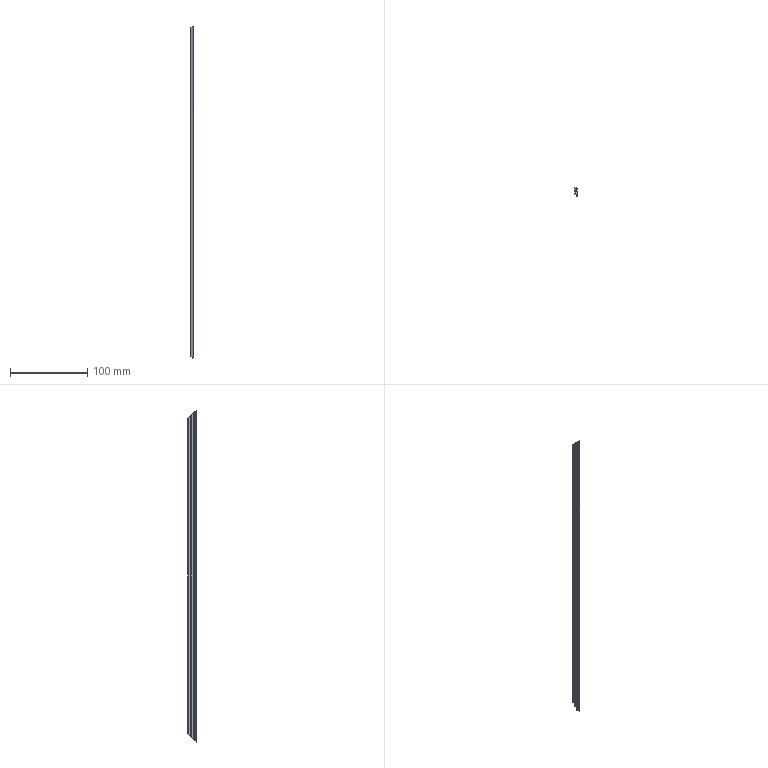Part | NX | features BREP 1 | 1 solid | 28 faces | box 3.587 x 11.224 x 429 mm | volume 9737 mm3 | plane 18 | cylinder 10 | commonest cylinder face diameters 0.4 x6 0.6 x2 1.942 x2
STEP:
#1=CARTESIAN_POINT('',(3.587,9.871,-204.628));
#2=VERTEX_POINT('',#1);
#3=CARTESIAN_POINT('',(3.287,9.567,-204.932));
#4=VERTEX_POINT('',#3);
#5=CARTESIAN_POINT('',(3.587,9.871,-204.628));
#6=CARTESIAN_POINT('',(3.589,9.693,-204.806));
#7=CARTESIAN_POINT('',(3.464,9.567,-204.932));
#8=CARTESIAN_POINT('',(3.287,9.567,-204.932));
#9=(BOUNDED_CURVE()B_SPLINE_CURVE(3,(#5,#6,#7,#8),.UNSPECIFIED.,.F.,.F.)B_SPLINE_CURVE_WITH_KNOTS((4,4),(4.699,6.283),.UNSPECIFIED.)CURVE()GEOMETRIC_REPRESENTATION_ITEM()RATIONAL_B_SPLINE_CURVE((1.,0.8015,0.8015,1.))REPRESENTATION_ITEM(''));
#10=EDGE_CURVE('',#2,#4,#9,.T.);
#11=ORIENTED_EDGE('',*,*,#10,.F.);
#12=CARTESIAN_POINT('',(3.587,9.871,204.628));
#13=VERTEX_POINT('',#12);
#14=CARTESIAN_POINT('',(3.587,9.871,214.5));
#15=DIRECTION('',(0.,0.,-1.));
#16=VECTOR('',#15,1000.);
#17=LINE('',#14,#16);
#18=EDGE_CURVE('',#13,#2,#17,.T.);
#19=ORIENTED_EDGE('',*,*,#18,.F.);
#20=CARTESIAN_POINT('',(3.287,9.567,204.932));
#21=VERTEX_POINT('',#20);
#22=CARTESIAN_POINT('',(3.287,9.567,204.932));
#23=CARTESIAN_POINT('',(3.464,9.567,204.932));
#24=CARTESIAN_POINT('',(3.589,9.693,204.806));
#25=CARTESIAN_POINT('',(3.587,9.871,204.628));
#26=(BOUNDED_CURVE()B_SPLINE_CURVE(3,(#22,#23,#24,#25),.UNSPECIFIED.,.F.,.F.)B_SPLINE_CURVE_WITH_KNOTS((4,4),(3.142,4.726),.UNSPECIFIED.)CURVE()GEOMETRIC_REPRESENTATION_ITEM()RATIONAL_B_SPLINE_CURVE((1.,0.8015,0.8015,1.))REPRESENTATION_ITEM(''));
#27=EDGE_CURVE('',#21,#13,#26,.T.);
#28=ORIENTED_EDGE('',*,*,#27,.F.);
#29=CARTESIAN_POINT('',(3.287,9.567,214.5));
#30=DIRECTION('',(0.,0.,-1.));
#31=VECTOR('',#30,1000.);
#32=LINE('',#29,#31);
#33=EDGE_CURVE('',#21,#4,#32,.T.);
#34=ORIENTED_EDGE('',*,*,#33,.T.);
#35=EDGE_LOOP('',(#11,#19,#28,#34));
#36=FACE_BOUND('',#35,.T.);
#37=CARTESIAN_POINT('',(3.287,9.867,214.5));
#38=DIRECTION('',(0.,0.,-1.));
#39=DIRECTION('',(-1.,0.,0.));
#40=AXIS2_PLACEMENT_3D('',#37,#38,#39);
#41=CYLINDRICAL_SURFACE('',#40,0.3);
#42=ADVANCED_FACE('',(#36),#41,.T.);
#43=CARTESIAN_POINT('',(3.447,10.36,-204.139));
#44=VERTEX_POINT('',#43);
#45=CARTESIAN_POINT('',(3.447,10.36,-204.139));
#46=CARTESIAN_POINT('',(3.536,10.211,-204.288));
#47=CARTESIAN_POINT('',(3.584,10.044,-204.455));
#48=CARTESIAN_POINT('',(3.587,9.871,-204.628));
#49=(BOUNDED_CURVE()B_SPLINE_CURVE(3,(#45,#46,#47,#48),.UNSPECIFIED.,.F.,.F.)B_SPLINE_CURVE_WITH_KNOTS((4,4),(4.169,4.699),.UNSPECIFIED.)CURVE()GEOMETRIC_REPRESENTATION_ITEM()RATIONAL_B_SPLINE_CURVE((1.,0.9767,0.9767,1.))REPRESENTATION_ITEM(''));
#50=EDGE_CURVE('',#44,#2,#49,.T.);
#51=ORIENTED_EDGE('',*,*,#50,.F.);
#52=CARTESIAN_POINT('',(3.447,10.36,204.139));
#53=VERTEX_POINT('',#52);
#54=CARTESIAN_POINT('',(3.447,10.36,214.5));
#55=DIRECTION('',(0.,0.,-1.));
#56=VECTOR('',#55,1000.);
#57=LINE('',#54,#56);
#58=EDGE_CURVE('',#53,#44,#57,.T.);
#59=ORIENTED_EDGE('',*,*,#58,.F.);
#60=CARTESIAN_POINT('',(3.587,9.871,204.628));
#61=CARTESIAN_POINT('',(3.584,10.044,204.455));
#62=CARTESIAN_POINT('',(3.536,10.211,204.288));
#63=CARTESIAN_POINT('',(3.447,10.36,204.139));
#64=(BOUNDED_CURVE()B_SPLINE_CURVE(3,(#60,#61,#62,#63),.UNSPECIFIED.,.F.,.F.)B_SPLINE_CURVE_WITH_KNOTS((4,4),(4.726,5.256),.UNSPECIFIED.)CURVE()GEOMETRIC_REPRESENTATION_ITEM()RATIONAL_B_SPLINE_CURVE((1.,0.9767,0.9767,1.))REPRESENTATION_ITEM(''));
#65=EDGE_CURVE('',#13,#53,#64,.T.);
#66=ORIENTED_EDGE('',*,*,#65,.F.);
#67=ORIENTED_EDGE('',*,*,#18,.T.);
#68=EDGE_LOOP('',(#51,#59,#66,#67));
#69=FACE_BOUND('',#68,.T.);
#70=CARTESIAN_POINT('',(2.616,9.857,214.5));
#71=DIRECTION('',(0.,0.,-1.));
#72=DIRECTION('',(-1.,0.,0.));
#73=AXIS2_PLACEMENT_3D('',#70,#71,#72);
#74=CYLINDRICAL_SURFACE('',#73,0.971);
#75=ADVANCED_FACE('',(#69),#74,.T.);
#76=CARTESIAN_POINT('',(0.2517,11.216,-203.283));
#77=VERTEX_POINT('',#76);
#78=CARTESIAN_POINT('',(-94.616,36.626,-177.873));
#79=DIRECTION('',(0.9352,-0.2505,-0.2505));
#80=VECTOR('',#79,1000.);
#81=LINE('',#78,#80);
#82=EDGE_CURVE('',#77,#44,#81,.T.);
#83=ORIENTED_EDGE('',*,*,#82,.F.);
#84=CARTESIAN_POINT('',(0.2517,11.216,203.283));
#85=VERTEX_POINT('',#84);
#86=CARTESIAN_POINT('',(0.2517,11.216,214.5));
#87=DIRECTION('',(0.,0.,-1.));
#88=VECTOR('',#87,1000.);
#89=LINE('',#86,#88);
#90=EDGE_CURVE('',#85,#77,#89,.T.);
#91=ORIENTED_EDGE('',*,*,#90,.F.);
#92=CARTESIAN_POINT('',(5.874,9.71,204.789));
#93=DIRECTION('',(-0.9352,0.2505,-0.2505));
#94=VECTOR('',#93,1000.);
#95=LINE('',#92,#94);
#96=EDGE_CURVE('',#53,#85,#95,.T.);
#97=ORIENTED_EDGE('',*,*,#96,.F.);
#98=ORIENTED_EDGE('',*,*,#58,.T.);
#99=EDGE_LOOP('',(#83,#91,#97,#98));
#100=FACE_BOUND('',#99,.T.);
#101=CARTESIAN_POINT('',(3.447,10.36,214.5));
#102=DIRECTION('',(-0.2587,-0.9659,0.));
#103=DIRECTION('',(-0.9659,0.2587,0.));
#104=AXIS2_PLACEMENT_3D('',#101,#102,#103);
#105=PLANE('',#104);
#106=ADVANCED_FACE('',(#100),#105,.F.);
#107=CARTESIAN_POINT('',(0.,11.022,-203.476));
#108=VERTEX_POINT('',#107);
#109=CARTESIAN_POINT('',(0.,11.022,-203.476));
#110=CARTESIAN_POINT('',(0.,11.165,-203.333));
#111=CARTESIAN_POINT('',(0.1135,11.253,-203.246));
#112=CARTESIAN_POINT('',(0.2517,11.216,-203.283));
#113=(BOUNDED_CURVE()B_SPLINE_CURVE(3,(#109,#110,#111,#112),.UNSPECIFIED.,.F.,.F.)B_SPLINE_CURVE_WITH_KNOTS((4,4),(1.571,3.403),.UNSPECIFIED.)CURVE()GEOMETRIC_REPRESENTATION_ITEM()RATIONAL_B_SPLINE_CURVE((1.,0.7392,0.7392,1.))REPRESENTATION_ITEM(''));
#114=EDGE_CURVE('',#108,#77,#113,.T.);
#115=ORIENTED_EDGE('',*,*,#114,.F.);
#116=CARTESIAN_POINT('',(0.,11.022,203.476));
#117=VERTEX_POINT('',#116);
#118=CARTESIAN_POINT('',(0.,11.022,214.5));
#119=DIRECTION('',(0.,0.,-1.));
#120=VECTOR('',#119,1000.);
#121=LINE('',#118,#120);
#122=EDGE_CURVE('',#117,#108,#121,.T.);
#123=ORIENTED_EDGE('',*,*,#122,.F.);
#124=CARTESIAN_POINT('',(0.2517,11.216,203.283));
#125=CARTESIAN_POINT('',(0.1135,11.253,203.246));
#126=CARTESIAN_POINT('',(0.,11.165,203.333));
#127=CARTESIAN_POINT('',(0.,11.022,203.476));
#128=(BOUNDED_CURVE()B_SPLINE_CURVE(3,(#124,#125,#126,#127),.UNSPECIFIED.,.F.,.F.)B_SPLINE_CURVE_WITH_KNOTS((4,4),(6.021,7.854),.UNSPECIFIED.)CURVE()GEOMETRIC_REPRESENTATION_ITEM()RATIONAL_B_SPLINE_CURVE((1.,0.7392,0.7392,1.))REPRESENTATION_ITEM(''));
#129=EDGE_CURVE('',#85,#117,#128,.T.);
#130=ORIENTED_EDGE('',*,*,#129,.F.);
#131=ORIENTED_EDGE('',*,*,#90,.T.);
#132=EDGE_LOOP('',(#115,#123,#130,#131));
#133=FACE_BOUND('',#132,.T.);
#134=CARTESIAN_POINT('',(0.2,11.022,214.5));
#135=DIRECTION('',(0.,0.,-1.));
#136=DIRECTION('',(-1.,0.,0.));
#137=AXIS2_PLACEMENT_3D('',#134,#135,#136);
#138=CYLINDRICAL_SURFACE('',#137,0.2);
#139=ADVANCED_FACE('',(#133),#138,.T.);
#140=CARTESIAN_POINT('',(0.,10.432,-204.067));
#141=VERTEX_POINT('',#140);
#142=CARTESIAN_POINT('',(0.,220.011,5.512));
#143=DIRECTION('',(0.,0.7071,0.7071));
#144=VECTOR('',#143,1000.);
#145=LINE('',#142,#144);
#146=EDGE_CURVE('',#141,#108,#145,.T.);
#147=ORIENTED_EDGE('',*,*,#146,.F.);
#148=CARTESIAN_POINT('',(0.,10.432,204.067));
#149=VERTEX_POINT('',#148);
#150=CARTESIAN_POINT('',(0.,10.432,214.5));
#151=DIRECTION('',(0.,0.,-1.));
#152=VECTOR('',#151,1000.);
#153=LINE('',#150,#152);
#154=EDGE_CURVE('',#149,#141,#153,.T.);
#155=ORIENTED_EDGE('',*,*,#154,.F.);
#156=CARTESIAN_POINT('',(0.,5.511,208.988));
#157=DIRECTION('',(0.,-0.7071,0.7071));
#158=VECTOR('',#157,1000.);
#159=LINE('',#156,#158);
#160=EDGE_CURVE('',#117,#149,#159,.T.);
#161=ORIENTED_EDGE('',*,*,#160,.F.);
#162=ORIENTED_EDGE('',*,*,#122,.T.);
#163=EDGE_LOOP('',(#147,#155,#161,#162));
#164=FACE_BOUND('',#163,.T.);
#165=CARTESIAN_POINT('',(0.,11.022,214.5));
#166=DIRECTION('',(1.,0.,0.));
#167=DIRECTION('',(0.,1.,0.));
#168=AXIS2_PLACEMENT_3D('',#165,#166,#167);
#169=PLANE('',#168);
#170=ADVANCED_FACE('',(#164),#169,.F.);
#171=CARTESIAN_POINT('',(0.1483,10.238,-204.26));
#172=VERTEX_POINT('',#171);
#173=CARTESIAN_POINT('',(0.1483,10.238,-204.26));
#174=CARTESIAN_POINT('',(0.05733,10.263,-204.236));
#175=CARTESIAN_POINT('',(0.,10.338,-204.161));
#176=CARTESIAN_POINT('',(0.,10.432,-204.067));
#177=(BOUNDED_CURVE()B_SPLINE_CURVE(3,(#173,#174,#175,#176),.UNSPECIFIED.,.F.,.F.)B_SPLINE_CURVE_WITH_KNOTS((4,4),(0.2616,1.571),.UNSPECIFIED.)CURVE()GEOMETRIC_REPRESENTATION_ITEM()RATIONAL_B_SPLINE_CURVE((1.,0.8622,0.8622,1.))REPRESENTATION_ITEM(''));
#178=EDGE_CURVE('',#172,#141,#177,.T.);
#179=ORIENTED_EDGE('',*,*,#178,.F.);
#180=CARTESIAN_POINT('',(0.1483,10.238,204.26));
#181=VERTEX_POINT('',#180);
#182=CARTESIAN_POINT('',(0.1483,10.238,214.5));
#183=DIRECTION('',(0.,0.,-1.));
#184=VECTOR('',#183,1000.);
#185=LINE('',#182,#184);
#186=EDGE_CURVE('',#181,#172,#185,.T.);
#187=ORIENTED_EDGE('',*,*,#186,.F.);
#188=CARTESIAN_POINT('',(0.,10.432,204.067));
#189=CARTESIAN_POINT('',(0.,10.338,204.161));
#190=CARTESIAN_POINT('',(0.05733,10.263,204.236));
#191=CARTESIAN_POINT('',(0.1483,10.238,204.26));
#192=(BOUNDED_CURVE()B_SPLINE_CURVE(3,(#188,#189,#190,#191),.UNSPECIFIED.,.F.,.F.)B_SPLINE_CURVE_WITH_KNOTS((4,4),(1.571,2.88),.UNSPECIFIED.)CURVE()GEOMETRIC_REPRESENTATION_ITEM()RATIONAL_B_SPLINE_CURVE((1.,0.8622,0.8622,1.))REPRESENTATION_ITEM(''));
#193=EDGE_CURVE('',#149,#181,#192,.T.);
#194=ORIENTED_EDGE('',*,*,#193,.F.);
#195=ORIENTED_EDGE('',*,*,#154,.T.);
#196=EDGE_LOOP('',(#179,#187,#194,#195));
#197=FACE_BOUND('',#196,.T.);
#198=CARTESIAN_POINT('',(0.2,10.432,214.5));
#199=DIRECTION('',(0.,0.,-1.));
#200=DIRECTION('',(-1.,0.,0.));
#201=AXIS2_PLACEMENT_3D('',#198,#199,#200);
#202=CYLINDRICAL_SURFACE('',#201,0.2);
#203=ADVANCED_FACE('',(#197),#202,.T.);
#204=CARTESIAN_POINT('',(0.854,10.05,-204.449));
#205=VERTEX_POINT('',#204);
#206=CARTESIAN_POINT('',(-97.905,36.489,-178.01));
#207=DIRECTION('',(-0.9352,0.2504,0.2504));
#208=VECTOR('',#207,1000.);
#209=LINE('',#206,#208);
#210=EDGE_CURVE('',#205,#172,#209,.T.);
#211=ORIENTED_EDGE('',*,*,#210,.F.);
#212=CARTESIAN_POINT('',(0.854,10.05,204.449));
#213=VERTEX_POINT('',#212);
#214=CARTESIAN_POINT('',(0.854,10.05,214.5));
#215=DIRECTION('',(0.,0.,-1.));
#216=VECTOR('',#215,1000.);
#217=LINE('',#214,#216);
#218=EDGE_CURVE('',#213,#205,#217,.T.);
#219=ORIENTED_EDGE('',*,*,#218,.F.);
#220=CARTESIAN_POINT('',(2.546,9.597,204.902));
#221=DIRECTION('',(0.9352,-0.2504,0.2504));
#222=VECTOR('',#221,1000.);
#223=LINE('',#220,#222);
#224=EDGE_CURVE('',#181,#213,#223,.T.);
#225=ORIENTED_EDGE('',*,*,#224,.F.);
#226=ORIENTED_EDGE('',*,*,#186,.T.);
#227=EDGE_LOOP('',(#211,#219,#225,#226));
#228=FACE_BOUND('',#227,.T.);
#229=CARTESIAN_POINT('',(0.1483,10.238,214.5));
#230=DIRECTION('',(0.2586,0.966,0.));
#231=DIRECTION('',(0.,0.,-1.));
#232=AXIS2_PLACEMENT_3D('',#229,#230,#231);
#233=PLANE('',#232);
#234=ADVANCED_FACE('',(#228),#233,.F.);
#235=CARTESIAN_POINT('',(1.256,6.926,-207.573));
#236=VERTEX_POINT('',#235);
#237=CARTESIAN_POINT('',(-25.866,217.806,3.307));
#238=DIRECTION('',(-0.09057,0.7042,0.7042));
#239=VECTOR('',#238,1000.);
#240=LINE('',#237,#239);
#241=EDGE_CURVE('',#236,#205,#240,.T.);
#242=ORIENTED_EDGE('',*,*,#241,.F.);
#243=CARTESIAN_POINT('',(1.256,6.926,207.573));
#244=VERTEX_POINT('',#243);
#245=CARTESIAN_POINT('',(1.256,6.926,214.5));
#246=DIRECTION('',(0.,0.,-1.));
#247=VECTOR('',#246,1000.);
#248=LINE('',#245,#247);
#249=EDGE_CURVE('',#244,#236,#248,.T.);
#250=ORIENTED_EDGE('',*,*,#249,.F.);
#251=CARTESIAN_POINT('',(1.495,5.065,209.433));
#252=DIRECTION('',(0.09057,-0.7042,0.7042));
#253=VECTOR('',#252,1000.);
#254=LINE('',#251,#253);
#255=EDGE_CURVE('',#213,#244,#254,.T.);
#256=ORIENTED_EDGE('',*,*,#255,.F.);
#257=ORIENTED_EDGE('',*,*,#218,.T.);
#258=EDGE_LOOP('',(#242,#250,#256,#257));
#259=FACE_BOUND('',#258,.T.);
#260=CARTESIAN_POINT('',(0.854,10.05,214.5));
#261=DIRECTION('',(0.9918,0.1276,0.));
#262=DIRECTION('',(0.,0.,-1.));
#263=AXIS2_PLACEMENT_3D('',#260,#261,#262);
#264=PLANE('',#263);
#265=ADVANCED_FACE('',(#259),#264,.F.);
#266=CARTESIAN_POINT('',(0.2517,7.195,-207.304));
#267=VERTEX_POINT('',#266);
#268=CARTESIAN_POINT('',(-97.576,33.385,-181.113));
#269=DIRECTION('',(0.9352,-0.2504,-0.2504));
#270=VECTOR('',#269,1000.);
#271=LINE('',#268,#270);
#272=EDGE_CURVE('',#267,#236,#271,.T.);
#273=ORIENTED_EDGE('',*,*,#272,.F.);
#274=CARTESIAN_POINT('',(0.2517,7.195,207.304));
#275=VERTEX_POINT('',#274);
#276=CARTESIAN_POINT('',(0.2517,7.195,214.5));
#277=DIRECTION('',(0.,0.,-1.));
#278=VECTOR('',#277,1000.);
#279=LINE('',#276,#278);
#280=EDGE_CURVE('',#275,#267,#279,.T.);
#281=ORIENTED_EDGE('',*,*,#280,.F.);
#282=CARTESIAN_POINT('',(2.878,6.492,208.007));
#283=DIRECTION('',(-0.9352,0.2504,-0.2504));
#284=VECTOR('',#283,1000.);
#285=LINE('',#282,#284);
#286=EDGE_CURVE('',#244,#275,#285,.T.);
#287=ORIENTED_EDGE('',*,*,#286,.F.);
#288=ORIENTED_EDGE('',*,*,#249,.T.);
#289=EDGE_LOOP('',(#273,#281,#287,#288));
#290=FACE_BOUND('',#289,.T.);
#291=CARTESIAN_POINT('',(1.256,6.926,214.5));
#292=DIRECTION('',(-0.2586,-0.966,0.));
#293=DIRECTION('',(-0.966,0.2586,0.));
#294=AXIS2_PLACEMENT_3D('',#291,#292,#293);
#295=PLANE('',#294);
#296=ADVANCED_FACE('',(#290),#295,.F.);
#297=CARTESIAN_POINT('',(0.,7.001,-207.497));
#298=VERTEX_POINT('',#297);
#299=CARTESIAN_POINT('',(0.,7.001,-207.497));
#300=CARTESIAN_POINT('',(0.,7.145,-207.354));
#301=CARTESIAN_POINT('',(0.1135,7.232,-207.267));
#302=CARTESIAN_POINT('',(0.2517,7.195,-207.304));
#303=(BOUNDED_CURVE()B_SPLINE_CURVE(3,(#299,#300,#301,#302),.UNSPECIFIED.,.F.,.F.)B_SPLINE_CURVE_WITH_KNOTS((4,4),(1.571,3.403),.UNSPECIFIED.)CURVE()GEOMETRIC_REPRESENTATION_ITEM()RATIONAL_B_SPLINE_CURVE((1.,0.7392,0.7392,1.))REPRESENTATION_ITEM(''));
#304=EDGE_CURVE('',#298,#267,#303,.T.);
#305=ORIENTED_EDGE('',*,*,#304,.F.);
#306=CARTESIAN_POINT('',(0.,7.001,207.497));
#307=VERTEX_POINT('',#306);
#308=CARTESIAN_POINT('',(0.,7.001,214.5));
#309=DIRECTION('',(0.,0.,-1.));
#310=VECTOR('',#309,1000.);
#311=LINE('',#308,#310);
#312=EDGE_CURVE('',#307,#298,#311,.T.);
#313=ORIENTED_EDGE('',*,*,#312,.F.);
#314=CARTESIAN_POINT('',(0.2517,7.195,207.304));
#315=CARTESIAN_POINT('',(0.1135,7.232,207.267));
#316=CARTESIAN_POINT('',(0.,7.145,207.354));
#317=CARTESIAN_POINT('',(0.,7.001,207.497));
#318=(BOUNDED_CURVE()B_SPLINE_CURVE(3,(#314,#315,#316,#317),.UNSPECIFIED.,.F.,.F.)B_SPLINE_CURVE_WITH_KNOTS((4,4),(6.022,7.854),.UNSPECIFIED.)CURVE()GEOMETRIC_REPRESENTATION_ITEM()RATIONAL_B_SPLINE_CURVE((1.,0.7392,0.7392,1.))REPRESENTATION_ITEM(''));
#319=EDGE_CURVE('',#275,#307,#318,.T.);
#320=ORIENTED_EDGE('',*,*,#319,.F.);
#321=ORIENTED_EDGE('',*,*,#280,.T.);
#322=EDGE_LOOP('',(#305,#313,#320,#321));
#323=FACE_BOUND('',#322,.T.);
#324=CARTESIAN_POINT('',(0.2,7.001,214.5));
#325=DIRECTION('',(0.,0.,-1.));
#326=DIRECTION('',(-1.,0.,0.));
#327=AXIS2_PLACEMENT_3D('',#324,#325,#326);
#328=CYLINDRICAL_SURFACE('',#327,0.2);
#329=ADVANCED_FACE('',(#323),#328,.T.);
#330=CARTESIAN_POINT('',(0.,6.41,-208.089));
#331=VERTEX_POINT('',#330);
#332=CARTESIAN_POINT('',(0.,218.,3.501));
#333=DIRECTION('',(0.,0.7071,0.7071));
#334=VECTOR('',#333,1000.);
#335=LINE('',#332,#334);
#336=EDGE_CURVE('',#331,#298,#335,.T.);
#337=ORIENTED_EDGE('',*,*,#336,.F.);
#338=CARTESIAN_POINT('',(0.,6.41,208.089));
#339=VERTEX_POINT('',#338);
#340=CARTESIAN_POINT('',(0.,6.41,214.5));
#341=DIRECTION('',(0.,0.,-1.));
#342=VECTOR('',#341,1000.);
#343=LINE('',#340,#342);
#344=EDGE_CURVE('',#339,#331,#343,.T.);
#345=ORIENTED_EDGE('',*,*,#344,.F.);
#346=CARTESIAN_POINT('',(0.,3.5,210.999));
#347=DIRECTION('',(0.,-0.7071,0.7071));
#348=VECTOR('',#347,1000.);
#349=LINE('',#346,#348);
#350=EDGE_CURVE('',#307,#339,#349,.T.);
#351=ORIENTED_EDGE('',*,*,#350,.F.);
#352=ORIENTED_EDGE('',*,*,#312,.T.);
#353=EDGE_LOOP('',(#337,#345,#351,#352));
#354=FACE_BOUND('',#353,.T.);
#355=CARTESIAN_POINT('',(0.,7.001,214.5));
#356=DIRECTION('',(1.,0.,0.));
#357=DIRECTION('',(0.,1.,0.));
#358=AXIS2_PLACEMENT_3D('',#355,#356,#357);
#359=PLANE('',#358);
#360=ADVANCED_FACE('',(#354),#359,.F.);
#361=CARTESIAN_POINT('',(0.1482,6.217,-208.282));
#362=VERTEX_POINT('',#361);
#363=CARTESIAN_POINT('',(0.1482,6.217,-208.282));
#364=CARTESIAN_POINT('',(0.0573,6.241,-208.258));
#365=CARTESIAN_POINT('',(0.,6.316,-208.183));
#366=CARTESIAN_POINT('',(0.,6.41,-208.089));
#367=(BOUNDED_CURVE()B_SPLINE_CURVE(3,(#363,#364,#365,#366),.UNSPECIFIED.,.F.,.F.)B_SPLINE_CURVE_WITH_KNOTS((4,4),(0.2619,1.571),.UNSPECIFIED.)CURVE()GEOMETRIC_REPRESENTATION_ITEM()RATIONAL_B_SPLINE_CURVE((1.,0.8623,0.8623,1.))REPRESENTATION_ITEM(''));
#368=EDGE_CURVE('',#362,#331,#367,.T.);
#369=ORIENTED_EDGE('',*,*,#368,.F.);
#370=CARTESIAN_POINT('',(0.1482,6.217,208.282));
#371=VERTEX_POINT('',#370);
#372=CARTESIAN_POINT('',(0.1482,6.217,214.5));
#373=DIRECTION('',(0.,0.,-1.));
#374=VECTOR('',#373,1000.);
#375=LINE('',#372,#374);
#376=EDGE_CURVE('',#371,#362,#375,.T.);
#377=ORIENTED_EDGE('',*,*,#376,.F.);
#378=CARTESIAN_POINT('',(0.,6.41,208.089));
#379=CARTESIAN_POINT('',(0.,6.316,208.183));
#380=CARTESIAN_POINT('',(0.0573,6.241,208.258));
#381=CARTESIAN_POINT('',(0.1482,6.217,208.282));
#382=(BOUNDED_CURVE()B_SPLINE_CURVE(3,(#378,#379,#380,#381),.UNSPECIFIED.,.F.,.F.)B_SPLINE_CURVE_WITH_KNOTS((4,4),(1.571,2.88),.UNSPECIFIED.)CURVE()GEOMETRIC_REPRESENTATION_ITEM()RATIONAL_B_SPLINE_CURVE((1.,0.8623,0.8623,1.))REPRESENTATION_ITEM(''));
#383=EDGE_CURVE('',#339,#371,#382,.T.);
#384=ORIENTED_EDGE('',*,*,#383,.F.);
#385=ORIENTED_EDGE('',*,*,#344,.T.);
#386=EDGE_LOOP('',(#369,#377,#384,#385));
#387=FACE_BOUND('',#386,.T.);
#388=CARTESIAN_POINT('',(0.2,6.41,214.5));
#389=DIRECTION('',(0.,0.,-1.));
#390=DIRECTION('',(-1.,0.,0.));
#391=AXIS2_PLACEMENT_3D('',#388,#389,#390);
#392=CYLINDRICAL_SURFACE('',#391,0.2);
#393=ADVANCED_FACE('',(#387),#392,.T.);
#394=CARTESIAN_POINT('',(1.39,5.884,-208.615));
#395=VERTEX_POINT('',#394);
#396=CARTESIAN_POINT('',(-98.949,32.783,-181.716));
#397=DIRECTION('',(-0.9351,0.2507,0.2507));
#398=VECTOR('',#397,1000.);
#399=LINE('',#396,#398);
#400=EDGE_CURVE('',#395,#362,#399,.T.);
#401=ORIENTED_EDGE('',*,*,#400,.F.);
#402=CARTESIAN_POINT('',(1.39,5.884,208.615));
#403=VERTEX_POINT('',#402);
#404=CARTESIAN_POINT('',(1.39,5.884,214.5));
#405=DIRECTION('',(0.,0.,-1.));
#406=VECTOR('',#405,1000.);
#407=LINE('',#404,#406);
#408=EDGE_CURVE('',#403,#395,#407,.T.);
#409=ORIENTED_EDGE('',*,*,#408,.F.);
#410=CARTESIAN_POINT('',(1.606,5.826,208.673));
#411=DIRECTION('',(0.9351,-0.2507,0.2507));
#412=VECTOR('',#411,1000.);
#413=LINE('',#410,#412);
#414=EDGE_CURVE('',#371,#403,#413,.T.);
#415=ORIENTED_EDGE('',*,*,#414,.F.);
#416=ORIENTED_EDGE('',*,*,#376,.T.);
#417=EDGE_LOOP('',(#401,#409,#415,#416));
#418=FACE_BOUND('',#417,.T.);
#419=CARTESIAN_POINT('',(0.1482,6.217,214.5));
#420=DIRECTION('',(0.2589,0.9659,0.));
#421=DIRECTION('',(0.,0.,-1.));
#422=AXIS2_PLACEMENT_3D('',#419,#420,#421);
#423=PLANE('',#422);
#424=ADVANCED_FACE('',(#418),#423,.F.);
#425=CARTESIAN_POINT('',(1.791,2.761,-211.738));
#426=VERTEX_POINT('',#425);
#427=CARTESIAN_POINT('',(-25.595,215.706,1.207));
#428=DIRECTION('',(-0.09057,0.7042,0.7042));
#429=VECTOR('',#428,1000.);
#430=LINE('',#427,#429);
#431=EDGE_CURVE('',#426,#395,#430,.T.);
#432=ORIENTED_EDGE('',*,*,#431,.F.);
#433=CARTESIAN_POINT('',(1.791,2.761,211.738));
#434=VERTEX_POINT('',#433);
#435=CARTESIAN_POINT('',(1.791,2.761,214.5));
#436=DIRECTION('',(0.,0.,-1.));
#437=VECTOR('',#436,1000.);
#438=LINE('',#435,#437);
#439=EDGE_CURVE('',#434,#426,#438,.T.);
#440=ORIENTED_EDGE('',*,*,#439,.F.);
#441=CARTESIAN_POINT('',(1.765,2.965,211.533));
#442=DIRECTION('',(0.09057,-0.7042,0.7042));
#443=VECTOR('',#442,1000.);
#444=LINE('',#441,#443);
#445=EDGE_CURVE('',#403,#434,#444,.T.);
#446=ORIENTED_EDGE('',*,*,#445,.F.);
#447=ORIENTED_EDGE('',*,*,#408,.T.);
#448=EDGE_LOOP('',(#432,#440,#446,#447));
#449=FACE_BOUND('',#448,.T.);
#450=CARTESIAN_POINT('',(1.39,5.884,214.5));
#451=DIRECTION('',(0.9918,0.1276,0.));
#452=DIRECTION('',(0.,0.,-1.));
#453=AXIS2_PLACEMENT_3D('',#450,#451,#452);
#454=PLANE('',#453);
#455=ADVANCED_FACE('',(#449),#454,.F.);
#456=CARTESIAN_POINT('',(0.2518,3.174,-211.325));
#457=VERTEX_POINT('',#456);
#458=CARTESIAN_POINT('',(-98.108,29.54,-184.959));
#459=DIRECTION('',(0.9351,-0.2506,-0.2506));
#460=VECTOR('',#459,1000.);
#461=LINE('',#458,#460);
#462=EDGE_CURVE('',#457,#426,#461,.T.);
#463=ORIENTED_EDGE('',*,*,#462,.F.);
#464=CARTESIAN_POINT('',(0.2518,3.174,211.325));
#465=VERTEX_POINT('',#464);
#466=CARTESIAN_POINT('',(0.2518,3.174,214.5));
#467=DIRECTION('',(0.,0.,-1.));
#468=VECTOR('',#467,1000.);
#469=LINE('',#466,#468);
#470=EDGE_CURVE('',#465,#457,#469,.T.);
#471=ORIENTED_EDGE('',*,*,#470,.F.);
#472=CARTESIAN_POINT('',(2.439,2.588,211.911));
#473=DIRECTION('',(-0.9351,0.2506,-0.2506));
#474=VECTOR('',#473,1000.);
#475=LINE('',#472,#474);
#476=EDGE_CURVE('',#434,#465,#475,.T.);
#477=ORIENTED_EDGE('',*,*,#476,.F.);
#478=ORIENTED_EDGE('',*,*,#439,.T.);
#479=EDGE_LOOP('',(#463,#471,#477,#478));
#480=FACE_BOUND('',#479,.T.);
#481=CARTESIAN_POINT('',(1.791,2.761,214.5));
#482=DIRECTION('',(-0.2589,-0.9659,0.));
#483=DIRECTION('',(-0.9659,0.2589,0.));
#484=AXIS2_PLACEMENT_3D('',#481,#482,#483);
#485=PLANE('',#484);
#486=ADVANCED_FACE('',(#480),#485,.F.);
#487=CARTESIAN_POINT('',(0.,2.981,-211.518));
#488=VERTEX_POINT('',#487);
#489=CARTESIAN_POINT('',(0.,2.981,-211.518));
#490=CARTESIAN_POINT('',(0.,3.124,-211.375));
#491=CARTESIAN_POINT('',(0.1135,3.211,-211.288));
#492=CARTESIAN_POINT('',(0.2518,3.174,-211.325));
#493=(BOUNDED_CURVE()B_SPLINE_CURVE(3,(#489,#490,#491,#492),.UNSPECIFIED.,.F.,.F.)B_SPLINE_CURVE_WITH_KNOTS((4,4),(1.571,3.403),.UNSPECIFIED.)CURVE()GEOMETRIC_REPRESENTATION_ITEM()RATIONAL_B_SPLINE_CURVE((1.,0.7391,0.7391,1.))REPRESENTATION_ITEM(''));
#494=EDGE_CURVE('',#488,#457,#493,.T.);
#495=ORIENTED_EDGE('',*,*,#494,.F.);
#496=CARTESIAN_POINT('',(0.,2.981,211.518));
#497=VERTEX_POINT('',#496);
#498=CARTESIAN_POINT('',(0.,2.981,214.5));
#499=DIRECTION('',(0.,0.,-1.));
#500=VECTOR('',#499,1000.);
#501=LINE('',#498,#500);
#502=EDGE_CURVE('',#497,#488,#501,.T.);
#503=ORIENTED_EDGE('',*,*,#502,.F.);
#504=CARTESIAN_POINT('',(0.2518,3.174,211.325));
#505=CARTESIAN_POINT('',(0.1135,3.211,211.288));
#506=CARTESIAN_POINT('',(0.,3.124,211.375));
#507=CARTESIAN_POINT('',(0.,2.981,211.518));
#508=(BOUNDED_CURVE()B_SPLINE_CURVE(3,(#504,#505,#506,#507),.UNSPECIFIED.,.F.,.F.)B_SPLINE_CURVE_WITH_KNOTS((4,4),(6.021,7.854),.UNSPECIFIED.)CURVE()GEOMETRIC_REPRESENTATION_ITEM()RATIONAL_B_SPLINE_CURVE((1.,0.7391,0.7391,1.))REPRESENTATION_ITEM(''));
#509=EDGE_CURVE('',#465,#497,#508,.T.);
#510=ORIENTED_EDGE('',*,*,#509,.F.);
#511=ORIENTED_EDGE('',*,*,#470,.T.);
#512=EDGE_LOOP('',(#495,#503,#510,#511));
#513=FACE_BOUND('',#512,.T.);
#514=CARTESIAN_POINT('',(0.2,2.981,214.5));
#515=DIRECTION('',(0.,0.,-1.));
#516=DIRECTION('',(-1.,0.,0.));
#517=AXIS2_PLACEMENT_3D('',#514,#515,#516);
#518=CYLINDRICAL_SURFACE('',#517,0.2);
#519=ADVANCED_FACE('',(#513),#518,.T.);
#520=CARTESIAN_POINT('',(0.,2.39,-212.109));
#521=VERTEX_POINT('',#520);
#522=CARTESIAN_POINT('',(0.,215.99,1.491));
#523=DIRECTION('',(0.,0.7071,0.7071));
#524=VECTOR('',#523,1000.);
#525=LINE('',#522,#524);
#526=EDGE_CURVE('',#521,#488,#525,.T.);
#527=ORIENTED_EDGE('',*,*,#526,.F.);
#528=CARTESIAN_POINT('',(0.,2.39,212.109));
#529=VERTEX_POINT('',#528);
#530=CARTESIAN_POINT('',(0.,2.39,214.5));
#531=DIRECTION('',(0.,0.,-1.));
#532=VECTOR('',#531,1000.);
#533=LINE('',#530,#532);
#534=EDGE_CURVE('',#529,#521,#533,.T.);
#535=ORIENTED_EDGE('',*,*,#534,.F.);
#536=CARTESIAN_POINT('',(0.,1.49,213.009));
#537=DIRECTION('',(0.,-0.7071,0.7071));
#538=VECTOR('',#537,1000.);
#539=LINE('',#536,#538);
#540=EDGE_CURVE('',#497,#529,#539,.T.);
#541=ORIENTED_EDGE('',*,*,#540,.F.);
#542=ORIENTED_EDGE('',*,*,#502,.T.);
#543=EDGE_LOOP('',(#527,#535,#541,#542));
#544=FACE_BOUND('',#543,.T.);
#545=CARTESIAN_POINT('',(0.,2.981,214.5));
#546=DIRECTION('',(1.,0.,0.));
#547=DIRECTION('',(0.,1.,0.));
#548=AXIS2_PLACEMENT_3D('',#545,#546,#547);
#549=PLANE('',#548);
#550=ADVANCED_FACE('',(#544),#549,.F.);
#551=CARTESIAN_POINT('',(0.1482,2.196,-212.302));
#552=VERTEX_POINT('',#551);
#553=CARTESIAN_POINT('',(0.1482,2.196,-212.302));
#554=CARTESIAN_POINT('',(0.05729,2.221,-212.278));
#555=CARTESIAN_POINT('',(0.,2.295,-212.203));
#556=CARTESIAN_POINT('',(0.,2.39,-212.109));
#557=(BOUNDED_CURVE()B_SPLINE_CURVE(3,(#553,#554,#555,#556),.UNSPECIFIED.,.F.,.F.)B_SPLINE_CURVE_WITH_KNOTS((4,4),(0.262,1.571),.UNSPECIFIED.)CURVE()GEOMETRIC_REPRESENTATION_ITEM()RATIONAL_B_SPLINE_CURVE((1.,0.8623,0.8623,1.))REPRESENTATION_ITEM(''));
#558=EDGE_CURVE('',#552,#521,#557,.T.);
#559=ORIENTED_EDGE('',*,*,#558,.F.);
#560=CARTESIAN_POINT('',(0.1482,2.196,212.302));
#561=VERTEX_POINT('',#560);
#562=CARTESIAN_POINT('',(0.1482,2.196,214.5));
#563=DIRECTION('',(0.,0.,-1.));
#564=VECTOR('',#563,1000.);
#565=LINE('',#562,#564);
#566=EDGE_CURVE('',#561,#552,#565,.T.);
#567=ORIENTED_EDGE('',*,*,#566,.F.);
#568=CARTESIAN_POINT('',(0.,2.39,212.109));
#569=CARTESIAN_POINT('',(0.,2.295,212.203));
#570=CARTESIAN_POINT('',(0.05729,2.221,212.278));
#571=CARTESIAN_POINT('',(0.1482,2.196,212.302));
#572=(BOUNDED_CURVE()B_SPLINE_CURVE(3,(#568,#569,#570,#571),.UNSPECIFIED.,.F.,.F.)B_SPLINE_CURVE_WITH_KNOTS((4,4),(1.571,2.88),.UNSPECIFIED.)CURVE()GEOMETRIC_REPRESENTATION_ITEM()RATIONAL_B_SPLINE_CURVE((1.,0.8623,0.8623,1.))REPRESENTATION_ITEM(''));
#573=EDGE_CURVE('',#529,#561,#572,.T.);
#574=ORIENTED_EDGE('',*,*,#573,.F.);
#575=ORIENTED_EDGE('',*,*,#534,.T.);
#576=EDGE_LOOP('',(#559,#567,#574,#575));
#577=FACE_BOUND('',#576,.T.);
#578=CARTESIAN_POINT('',(0.2,2.39,214.5));
#579=DIRECTION('',(0.,0.,-1.));
#580=DIRECTION('',(-1.,0.,0.));
#581=AXIS2_PLACEMENT_3D('',#578,#579,#580);
#582=CYLINDRICAL_SURFACE('',#581,0.2);
#583=ADVANCED_FACE('',(#577),#582,.T.);
#584=CARTESIAN_POINT('',(1.925,1.72,-212.779));
#585=VERTEX_POINT('',#584);
#586=CARTESIAN_POINT('',(-99.901,29.022,-185.477));
#587=DIRECTION('',(-0.935,0.2507,0.2507));
#588=VECTOR('',#587,1000.);
#589=LINE('',#586,#588);
#590=EDGE_CURVE('',#585,#552,#589,.T.);
#591=ORIENTED_EDGE('',*,*,#590,.F.);
#592=CARTESIAN_POINT('',(1.925,1.72,212.779));
#593=VERTEX_POINT('',#592);
#594=CARTESIAN_POINT('',(1.925,1.72,214.5));
#595=DIRECTION('',(0.,0.,-1.));
#596=VECTOR('',#595,1000.);
#597=LINE('',#594,#596);
#598=EDGE_CURVE('',#593,#585,#597,.T.);
#599=ORIENTED_EDGE('',*,*,#598,.F.);
#600=CARTESIAN_POINT('',(0.6633,2.058,212.441));
#601=DIRECTION('',(0.935,-0.2507,0.2507));
#602=VECTOR('',#601,1000.);
#603=LINE('',#600,#602);
#604=EDGE_CURVE('',#561,#593,#603,.T.);
#605=ORIENTED_EDGE('',*,*,#604,.F.);
#606=ORIENTED_EDGE('',*,*,#566,.T.);
#607=EDGE_LOOP('',(#591,#599,#605,#606));
#608=FACE_BOUND('',#607,.T.);
#609=CARTESIAN_POINT('',(0.1482,2.196,214.5));
#610=DIRECTION('',(0.259,0.9659,0.));
#611=DIRECTION('',(0.,0.,-1.));
#612=AXIS2_PLACEMENT_3D('',#609,#610,#611);
#613=PLANE('',#612);
#614=ADVANCED_FACE('',(#608),#613,.F.);
#615=CARTESIAN_POINT('',(2.108,0.3017,-214.197));
#616=VERTEX_POINT('',#615);
#617=CARTESIAN_POINT('',(-25.326,213.607,-0.8918));
#618=DIRECTION('',(-0.09057,0.7042,0.7042));
#619=VECTOR('',#618,1000.);
#620=LINE('',#617,#619);
#621=EDGE_CURVE('',#616,#585,#620,.T.);
#622=ORIENTED_EDGE('',*,*,#621,.F.);
#623=CARTESIAN_POINT('',(2.108,0.3017,214.197));
#624=VERTEX_POINT('',#623);
#625=CARTESIAN_POINT('',(2.108,0.3017,214.5));
#626=DIRECTION('',(0.,0.,-1.));
#627=VECTOR('',#626,1000.);
#628=LINE('',#625,#627);
#629=EDGE_CURVE('',#624,#616,#628,.T.);
#630=ORIENTED_EDGE('',*,*,#629,.F.);
#631=CARTESIAN_POINT('',(2.035,0.8664,213.632));
#632=DIRECTION('',(0.09057,-0.7042,0.7042));
#633=VECTOR('',#632,1000.);
#634=LINE('',#631,#633);
#635=EDGE_CURVE('',#593,#624,#634,.T.);
#636=ORIENTED_EDGE('',*,*,#635,.F.);
#637=ORIENTED_EDGE('',*,*,#598,.T.);
#638=EDGE_LOOP('',(#622,#630,#636,#637));
#639=FACE_BOUND('',#638,.T.);
#640=CARTESIAN_POINT('',(1.925,1.72,214.5));
#641=DIRECTION('',(0.9918,0.1276,0.));
#642=DIRECTION('',(0.,0.,-1.));
#643=AXIS2_PLACEMENT_3D('',#640,#641,#642);
#644=PLANE('',#643);
#645=ADVANCED_FACE('',(#639),#644,.F.);
#646=ORIENTED_EDGE('',*,*,#629,.T.);
#647=CARTESIAN_POINT('',(3.447,0.2347,-214.264));
#648=VERTEX_POINT('',#647);
#649=CARTESIAN_POINT('',(3.447,0.2347,-214.264));
#650=CARTESIAN_POINT('',(3.032,-0.1233,-214.622));
#651=CARTESIAN_POINT('',(2.485,-0.0959,-214.595));
#652=CARTESIAN_POINT('',(2.108,0.3017,-214.197));
#653=(BOUNDED_CURVE()B_SPLINE_CURVE(3,(#649,#650,#651,#652),.UNSPECIFIED.,.F.,.F.)B_SPLINE_CURVE_WITH_KNOTS((4,4),(5.571,7.095),.UNSPECIFIED.)CURVE()GEOMETRIC_REPRESENTATION_ITEM()RATIONAL_B_SPLINE_CURVE((1.,0.8156,0.8156,1.))REPRESENTATION_ITEM(''));
#654=EDGE_CURVE('',#648,#616,#653,.T.);
#655=ORIENTED_EDGE('',*,*,#654,.F.);
#656=CARTESIAN_POINT('',(3.447,0.2347,214.264));
#657=VERTEX_POINT('',#656);
#658=CARTESIAN_POINT('',(3.447,0.2347,214.5));
#659=DIRECTION('',(0.,0.,-1.));
#660=VECTOR('',#659,1000.);
#661=LINE('',#658,#660);
#662=EDGE_CURVE('',#657,#648,#661,.T.);
#663=ORIENTED_EDGE('',*,*,#662,.F.);
#664=CARTESIAN_POINT('',(2.108,0.3017,214.197));
#665=CARTESIAN_POINT('',(2.485,-0.0959,214.595));
#666=CARTESIAN_POINT('',(3.032,-0.1233,214.622));
#667=CARTESIAN_POINT('',(3.447,0.2347,214.264));
#668=(BOUNDED_CURVE()B_SPLINE_CURVE(3,(#664,#665,#666,#667),.UNSPECIFIED.,.F.,.F.)B_SPLINE_CURVE_WITH_KNOTS((4,4),(2.33,3.854),.UNSPECIFIED.)CURVE()GEOMETRIC_REPRESENTATION_ITEM()RATIONAL_B_SPLINE_CURVE((1.,0.8156,0.8156,1.))REPRESENTATION_ITEM(''));
#669=EDGE_CURVE('',#624,#657,#668,.T.);
#670=ORIENTED_EDGE('',*,*,#669,.F.);
#671=EDGE_LOOP('',(#646,#655,#663,#670));
#672=FACE_BOUND('',#671,.T.);
#673=CARTESIAN_POINT('',(2.812,0.9697,214.5));
#674=DIRECTION('',(0.,0.,-1.));
#675=DIRECTION('',(-1.,0.,0.));
#676=AXIS2_PLACEMENT_3D('',#673,#674,#675);
#677=CYLINDRICAL_SURFACE('',#676,0.971);
#678=ADVANCED_FACE('',(#672),#677,.T.);
#679=CARTESIAN_POINT('',(3.447,5.067,-209.432));
#680=VERTEX_POINT('',#679);
#681=CARTESIAN_POINT('',(3.447,214.617,0.1179));
#682=DIRECTION('',(0.,-0.7071,-0.7071));
#683=VECTOR('',#682,1000.);
#684=LINE('',#681,#683);
#685=EDGE_CURVE('',#680,#648,#684,.T.);
#686=ORIENTED_EDGE('',*,*,#685,.F.);
#687=CARTESIAN_POINT('',(3.447,5.067,209.432));
#688=VERTEX_POINT('',#687);
#689=CARTESIAN_POINT('',(3.447,5.067,214.5));
#690=DIRECTION('',(0.,0.,-1.));
#691=VECTOR('',#690,1000.);
#692=LINE('',#689,#691);
#693=EDGE_CURVE('',#688,#680,#692,.T.);
#694=ORIENTED_EDGE('',*,*,#693,.F.);
#695=CARTESIAN_POINT('',(3.447,0.1167,214.382));
#696=DIRECTION('',(0.,0.7071,-0.7071));
#697=VECTOR('',#696,1000.);
#698=LINE('',#695,#697);
#699=EDGE_CURVE('',#657,#688,#698,.T.);
#700=ORIENTED_EDGE('',*,*,#699,.F.);
#701=ORIENTED_EDGE('',*,*,#662,.T.);
#702=EDGE_LOOP('',(#686,#694,#700,#701));
#703=FACE_BOUND('',#702,.T.);
#704=CARTESIAN_POINT('',(3.447,0.2347,214.5));
#705=DIRECTION('',(-1.,0.,0.));
#706=DIRECTION('',(0.,0.,1.));
#707=AXIS2_PLACEMENT_3D('',#704,#705,#706);
#708=PLANE('',#707);
#709=ADVANCED_FACE('',(#703),#708,.F.);
#710=CARTESIAN_POINT('',(3.147,5.367,-209.132));
#711=VERTEX_POINT('',#710);
#712=CARTESIAN_POINT('',(3.147,5.367,-209.132));
#713=CARTESIAN_POINT('',(3.322,5.367,-209.132));
#714=CARTESIAN_POINT('',(3.447,5.242,-209.256));
#715=CARTESIAN_POINT('',(3.447,5.067,-209.432));
#716=(BOUNDED_CURVE()B_SPLINE_CURVE(3,(#712,#713,#714,#715),.UNSPECIFIED.,.F.,.F.)B_SPLINE_CURVE_WITH_KNOTS((4,4),(3.142,4.712),.UNSPECIFIED.)CURVE()GEOMETRIC_REPRESENTATION_ITEM()RATIONAL_B_SPLINE_CURVE((1.,0.8047,0.8047,1.))REPRESENTATION_ITEM(''));
#717=EDGE_CURVE('',#711,#680,#716,.T.);
#718=ORIENTED_EDGE('',*,*,#717,.F.);
#719=CARTESIAN_POINT('',(3.147,5.367,209.132));
#720=VERTEX_POINT('',#719);
#721=CARTESIAN_POINT('',(3.147,5.367,214.5));
#722=DIRECTION('',(0.,0.,-1.));
#723=VECTOR('',#722,1000.);
#724=LINE('',#721,#723);
#725=EDGE_CURVE('',#720,#711,#724,.T.);
#726=ORIENTED_EDGE('',*,*,#725,.F.);
#727=CARTESIAN_POINT('',(3.447,5.067,209.432));
#728=CARTESIAN_POINT('',(3.447,5.242,209.256));
#729=CARTESIAN_POINT('',(3.322,5.367,209.132));
#730=CARTESIAN_POINT('',(3.147,5.367,209.132));
#731=(BOUNDED_CURVE()B_SPLINE_CURVE(3,(#727,#728,#729,#730),.UNSPECIFIED.,.F.,.F.)B_SPLINE_CURVE_WITH_KNOTS((4,4),(4.712,6.283),.UNSPECIFIED.)CURVE()GEOMETRIC_REPRESENTATION_ITEM()RATIONAL_B_SPLINE_CURVE((1.,0.8047,0.8047,1.))REPRESENTATION_ITEM(''));
#732=EDGE_CURVE('',#688,#720,#731,.T.);
#733=ORIENTED_EDGE('',*,*,#732,.F.);
#734=ORIENTED_EDGE('',*,*,#693,.T.);
#735=EDGE_LOOP('',(#718,#726,#733,#734));
#736=FACE_BOUND('',#735,.T.);
#737=CARTESIAN_POINT('',(3.147,5.067,214.5));
#738=DIRECTION('',(0.,0.,-1.));
#739=DIRECTION('',(-1.,0.,0.));
#740=AXIS2_PLACEMENT_3D('',#737,#738,#739);
#741=CYLINDRICAL_SURFACE('',#740,0.3);
#742=ADVANCED_FACE('',(#736),#741,.T.);
#743=CARTESIAN_POINT('',(3.,5.367,-209.132));
#744=VERTEX_POINT('',#743);
#745=CARTESIAN_POINT('',(3.147,5.367,-209.132));
#746=DIRECTION('',(1.,0.,0.));
#747=VECTOR('',#746,1000.);
#748=LINE('',#745,#747);
#749=EDGE_CURVE('',#744,#711,#748,.T.);
#750=ORIENTED_EDGE('',*,*,#749,.F.);
#751=CARTESIAN_POINT('',(3.,5.367,209.132));
#752=VERTEX_POINT('',#751);
#753=CARTESIAN_POINT('',(3.,5.367,214.5));
#754=DIRECTION('',(0.,0.,-1.));
#755=VECTOR('',#754,1000.);
#756=LINE('',#753,#755);
#757=EDGE_CURVE('',#752,#744,#756,.T.);
#758=ORIENTED_EDGE('',*,*,#757,.F.);
#759=CARTESIAN_POINT('',(3.147,5.367,209.132));
#760=DIRECTION('',(-1.,0.,0.));
#761=VECTOR('',#760,1000.);
#762=LINE('',#759,#761);
#763=EDGE_CURVE('',#720,#752,#762,.T.);
#764=ORIENTED_EDGE('',*,*,#763,.F.);
#765=ORIENTED_EDGE('',*,*,#725,.T.);
#766=EDGE_LOOP('',(#750,#758,#764,#765));
#767=FACE_BOUND('',#766,.T.);
#768=CARTESIAN_POINT('',(3.147,5.367,214.5));
#769=DIRECTION('',(0.,-1.,0.));
#770=DIRECTION('',(0.,0.,-1.));
#771=AXIS2_PLACEMENT_3D('',#768,#769,#770);
#772=PLANE('',#771);
#773=ADVANCED_FACE('',(#767),#772,.F.);
#774=CARTESIAN_POINT('',(3.,9.567,-204.932));
#775=VERTEX_POINT('',#774);
#776=CARTESIAN_POINT('',(3.,217.183,2.684));
#777=DIRECTION('',(0.,-0.7071,-0.7071));
#778=VECTOR('',#777,1000.);
#779=LINE('',#776,#778);
#780=EDGE_CURVE('',#775,#744,#779,.T.);
#781=ORIENTED_EDGE('',*,*,#780,.F.);
#782=CARTESIAN_POINT('',(3.,9.567,204.932));
#783=VERTEX_POINT('',#782);
#784=CARTESIAN_POINT('',(3.,9.567,214.5));
#785=DIRECTION('',(0.,0.,-1.));
#786=VECTOR('',#785,1000.);
#787=LINE('',#784,#786);
#788=EDGE_CURVE('',#783,#775,#787,.T.);
#789=ORIENTED_EDGE('',*,*,#788,.F.);
#790=CARTESIAN_POINT('',(3.,2.683,211.816));
#791=DIRECTION('',(0.,0.7071,-0.7071));
#792=VECTOR('',#791,1000.);
#793=LINE('',#790,#792);
#794=EDGE_CURVE('',#752,#783,#793,.T.);
#795=ORIENTED_EDGE('',*,*,#794,.F.);
#796=ORIENTED_EDGE('',*,*,#757,.T.);
#797=EDGE_LOOP('',(#781,#789,#795,#796));
#798=FACE_BOUND('',#797,.T.);
#799=CARTESIAN_POINT('',(3.,5.367,214.5));
#800=DIRECTION('',(-1.,0.,0.));
#801=DIRECTION('',(0.,0.,1.));
#802=AXIS2_PLACEMENT_3D('',#799,#800,#801);
#803=PLANE('',#802);
#804=ADVANCED_FACE('',(#798),#803,.F.);
#805=CARTESIAN_POINT('',(3.,9.567,-204.932));
#806=DIRECTION('',(-1.,0.,0.));
#807=VECTOR('',#806,1000.);
#808=LINE('',#805,#807);
#809=EDGE_CURVE('',#4,#775,#808,.T.);
#810=ORIENTED_EDGE('',*,*,#809,.F.);
#811=ORIENTED_EDGE('',*,*,#33,.F.);
#812=CARTESIAN_POINT('',(3.,9.567,204.932));
#813=DIRECTION('',(1.,0.,0.));
#814=VECTOR('',#813,1000.);
#815=LINE('',#812,#814);
#816=EDGE_CURVE('',#783,#21,#815,.T.);
#817=ORIENTED_EDGE('',*,*,#816,.F.);
#818=ORIENTED_EDGE('',*,*,#788,.T.);
#819=EDGE_LOOP('',(#810,#811,#817,#818));
#820=FACE_BOUND('',#819,.T.);
#821=CARTESIAN_POINT('',(3.,9.567,214.5));
#822=DIRECTION('',(0.,1.,0.));
#823=DIRECTION('',(1.,0.,0.));
#824=AXIS2_PLACEMENT_3D('',#821,#822,#823);
#825=PLANE('',#824);
#826=ADVANCED_FACE('',(#820),#825,.F.);
#827=ORIENTED_EDGE('',*,*,#65,.T.);
#828=ORIENTED_EDGE('',*,*,#96,.T.);
#829=ORIENTED_EDGE('',*,*,#129,.T.);
#830=ORIENTED_EDGE('',*,*,#160,.T.);
#831=ORIENTED_EDGE('',*,*,#193,.T.);
#832=ORIENTED_EDGE('',*,*,#224,.T.);
#833=ORIENTED_EDGE('',*,*,#255,.T.);
#834=ORIENTED_EDGE('',*,*,#286,.T.);
#835=ORIENTED_EDGE('',*,*,#319,.T.);
#836=ORIENTED_EDGE('',*,*,#350,.T.);
#837=ORIENTED_EDGE('',*,*,#383,.T.);
#838=ORIENTED_EDGE('',*,*,#414,.T.);
#839=ORIENTED_EDGE('',*,*,#445,.T.);
#840=ORIENTED_EDGE('',*,*,#476,.T.);
#841=ORIENTED_EDGE('',*,*,#509,.T.);
#842=ORIENTED_EDGE('',*,*,#540,.T.);
#843=ORIENTED_EDGE('',*,*,#573,.T.);
#844=ORIENTED_EDGE('',*,*,#604,.T.);
#845=ORIENTED_EDGE('',*,*,#635,.T.);
#846=ORIENTED_EDGE('',*,*,#669,.T.);
#847=ORIENTED_EDGE('',*,*,#699,.T.);
#848=ORIENTED_EDGE('',*,*,#732,.T.);
#849=ORIENTED_EDGE('',*,*,#763,.T.);
#850=ORIENTED_EDGE('',*,*,#794,.T.);
#851=ORIENTED_EDGE('',*,*,#816,.T.);
#852=ORIENTED_EDGE('',*,*,#27,.T.);
#853=EDGE_LOOP('',(#827,#828,#829,#830,#831,#832,#833,#834,#835,#836,#837,#838,#839,#840,#841,#842,#843,#844,#845,#846,#847,#848,#849,#850,#851,#852));
#854=FACE_BOUND('',#853,.T.);
#855=CARTESIAN_POINT('',(3.587,-0.001213,214.5));
#856=DIRECTION('',(0.,0.7071,0.7071));
#857=DIRECTION('',(1.,0.,0.));
#858=AXIS2_PLACEMENT_3D('',#855,#856,#857);
#859=PLANE('',#858);
#860=ADVANCED_FACE('',(#854),#859,.T.);
#861=ORIENTED_EDGE('',*,*,#10,.T.);
#862=ORIENTED_EDGE('',*,*,#809,.T.);
#863=ORIENTED_EDGE('',*,*,#780,.T.);
#864=ORIENTED_EDGE('',*,*,#749,.T.);
#865=ORIENTED_EDGE('',*,*,#717,.T.);
#866=ORIENTED_EDGE('',*,*,#685,.T.);
#867=ORIENTED_EDGE('',*,*,#654,.T.);
#868=ORIENTED_EDGE('',*,*,#621,.T.);
#869=ORIENTED_EDGE('',*,*,#590,.T.);
#870=ORIENTED_EDGE('',*,*,#558,.T.);
#871=ORIENTED_EDGE('',*,*,#526,.T.);
#872=ORIENTED_EDGE('',*,*,#494,.T.);
#873=ORIENTED_EDGE('',*,*,#462,.T.);
#874=ORIENTED_EDGE('',*,*,#431,.T.);
#875=ORIENTED_EDGE('',*,*,#400,.T.);
#876=ORIENTED_EDGE('',*,*,#368,.T.);
#877=ORIENTED_EDGE('',*,*,#336,.T.);
#878=ORIENTED_EDGE('',*,*,#304,.T.);
#879=ORIENTED_EDGE('',*,*,#272,.T.);
#880=ORIENTED_EDGE('',*,*,#241,.T.);
#881=ORIENTED_EDGE('',*,*,#210,.T.);
#882=ORIENTED_EDGE('',*,*,#178,.T.);
#883=ORIENTED_EDGE('',*,*,#146,.T.);
#884=ORIENTED_EDGE('',*,*,#114,.T.);
#885=ORIENTED_EDGE('',*,*,#82,.T.);
#886=ORIENTED_EDGE('',*,*,#50,.T.);
#887=EDGE_LOOP('',(#861,#862,#863,#864,#865,#866,#867,#868,#869,#870,#871,#872,#873,#874,#875,#876,#877,#878,#879,#880,#881,#882,#883,#884,#885,#886));
#888=FACE_BOUND('',#887,.T.);
#889=CARTESIAN_POINT('',(3.587,-0.001213,-214.5));
#890=DIRECTION('',(0.,0.7071,-0.7071));
#891=DIRECTION('',(-1.,0.,0.));
#892=AXIS2_PLACEMENT_3D('',#889,#890,#891);
#893=PLANE('',#892);
#894=ADVANCED_FACE('',(#888),#893,.T.);
#895=CLOSED_SHELL('',(#42,#75,#106,#139,#170,#203,#234,#265,#296,#329,#360,#393,#424,#455,#486,#519,#550,#583,#614,#645,#678,#709,#742,#773,#804,#826,#860,#894));
#896=MANIFOLD_SOLID_BREP('',#895);
#897=(LENGTH_UNIT()NAMED_UNIT(*)SI_UNIT(.MILLI.,.METRE.));
#898=UNCERTAINTY_MEASURE_WITH_UNIT(LENGTH_MEASURE(0.00001),#897,'','');
#899=(NAMED_UNIT(*)PLANE_ANGLE_UNIT()SI_UNIT($,.RADIAN.));
#900=(NAMED_UNIT(*)SI_UNIT($,.STERADIAN.)SOLID_ANGLE_UNIT());
#901=(GEOMETRIC_REPRESENTATION_CONTEXT(3)GLOBAL_UNCERTAINTY_ASSIGNED_CONTEXT((#898))GLOBAL_UNIT_ASSIGNED_CONTEXT((#897,#899,#900))REPRESENTATION_CONTEXT('',''));
#902=ADVANCED_BREP_SHAPE_REPRESENTATION('',(#896),#901);